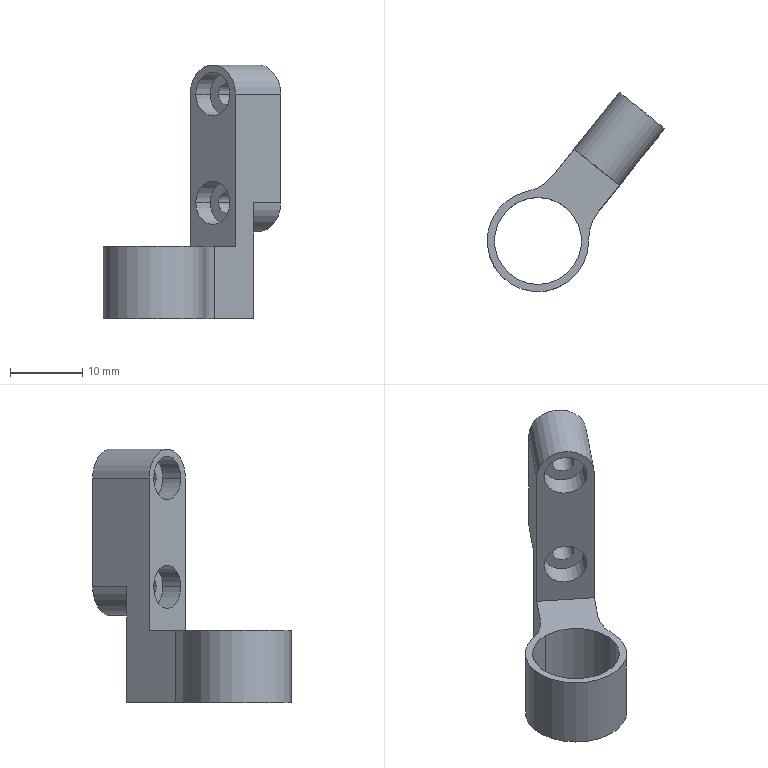Part | SolidWorks | features BaseBody 1 | 1 solid | 24 faces | box 24.488 x 27.462 x 35 mm | volume 2773 mm3 | cylinder 15 | plane 9 | commonest cylinder face diameters 3 x4 6 x4 12 x4 8 x2 14 x1
STEP:
#1=CARTESIAN_POINT('',(534.952,-197.215,297.045));
#2=VERTEX_POINT('',#1);
#3=CARTESIAN_POINT('',(534.952,-209.215,297.045));
#4=VERTEX_POINT('',#3);
#5=CARTESIAN_POINT('',(534.952,-203.215,297.045));
#6=DIRECTION('',(0.000000001,-0.000000003,1.));
#7=DIRECTION('',(0.,-1.,-0.000000003));
#8=AXIS2_PLACEMENT_3D('',#5,#6,#7);
#9=CIRCLE('',#8,6.);
#10=EDGE_CURVE('',#2,#4,#9,.T.);
#11=ORIENTED_EDGE('',*,*,#10,.F.);
#12=CARTESIAN_POINT('',(534.952,-197.215,307.045));
#13=VERTEX_POINT('',#12);
#14=CARTESIAN_POINT('',(534.952,-197.215,307.045));
#15=DIRECTION('',(0.000000001,-0.000000003,1.));
#16=VECTOR('',#15,1000.);
#17=LINE('',#14,#16);
#18=EDGE_CURVE('',#2,#13,#17,.T.);
#19=ORIENTED_EDGE('',*,*,#18,.T.);
#20=CARTESIAN_POINT('',(534.952,-209.215,307.045));
#21=VERTEX_POINT('',#20);
#22=CARTESIAN_POINT('',(534.952,-203.215,307.045));
#23=DIRECTION('',(-0.000000001,0.000000003,-1.));
#24=DIRECTION('',(0.,-1.,-0.000000003));
#25=AXIS2_PLACEMENT_3D('',#22,#23,#24);
#26=CIRCLE('',#25,6.);
#27=EDGE_CURVE('',#21,#13,#26,.T.);
#28=ORIENTED_EDGE('',*,*,#27,.F.);
#29=CARTESIAN_POINT('',(534.952,-209.215,307.045));
#30=DIRECTION('',(0.000000001,-0.000000003,1.));
#31=VECTOR('',#30,1000.);
#32=LINE('',#29,#31);
#33=EDGE_CURVE('',#4,#21,#32,.T.);
#34=ORIENTED_EDGE('',*,*,#33,.F.);
#35=EDGE_LOOP('',(#11,#19,#28,#34));
#36=FACE_OUTER_BOUND('',#35,.T.);
#37=CARTESIAN_POINT('',(534.952,-203.215,307.045));
#38=DIRECTION('',(0.000000001,-0.000000003,1.));
#39=DIRECTION('',(0.,-1.,-0.000000003));
#40=AXIS2_PLACEMENT_3D('',#37,#38,#39);
#41=CYLINDRICAL_SURFACE('',#40,6.);
#42=ADVANCED_FACE('',(#36),#41,.F.);
#43=CARTESIAN_POINT('',(542.711,-188.709,313.045));
#44=VERTEX_POINT('',#43);
#45=CARTESIAN_POINT('',(547.397,-192.455,313.045));
#46=VERTEX_POINT('',#45);
#47=CARTESIAN_POINT('',(545.054,-190.582,313.045));
#48=DIRECTION('',(-0.6245,-0.781,-0.000000002));
#49=DIRECTION('',(0.781,-0.6245,0.));
#50=AXIS2_PLACEMENT_3D('',#47,#48,#49);
#51=CIRCLE('',#50,3.);
#52=EDGE_CURVE('',#44,#46,#51,.T.);
#53=ORIENTED_EDGE('',*,*,#52,.F.);
#54=CARTESIAN_POINT('',(540.728,-191.188,313.045));
#55=VERTEX_POINT('',#54);
#56=CARTESIAN_POINT('',(541.719,-189.948,313.045));
#57=DIRECTION('',(-0.6245,-0.781,-0.000000002));
#58=VECTOR('',#57,1000.);
#59=LINE('',#56,#58);
#60=EDGE_CURVE('',#44,#55,#59,.T.);
#61=ORIENTED_EDGE('',*,*,#60,.T.);
#62=CARTESIAN_POINT('',(545.414,-194.935,313.045));
#63=VERTEX_POINT('',#62);
#64=CARTESIAN_POINT('',(543.071,-193.062,313.045));
#65=DIRECTION('',(0.6245,0.781,0.000000002));
#66=DIRECTION('',(0.781,-0.6245,0.));
#67=AXIS2_PLACEMENT_3D('',#64,#65,#66);
#68=CIRCLE('',#67,3.);
#69=EDGE_CURVE('',#63,#55,#68,.T.);
#70=ORIENTED_EDGE('',*,*,#69,.F.);
#71=CARTESIAN_POINT('',(546.405,-193.695,313.045));
#72=DIRECTION('',(-0.6245,-0.781,-0.000000002));
#73=VECTOR('',#72,1000.);
#74=LINE('',#71,#73);
#75=EDGE_CURVE('',#46,#63,#74,.T.);
#76=ORIENTED_EDGE('',*,*,#75,.F.);
#77=EDGE_LOOP('',(#53,#61,#70,#76));
#78=FACE_OUTER_BOUND('',#77,.T.);
#79=CARTESIAN_POINT('',(544.062,-191.822,313.045));
#80=DIRECTION('',(-0.6245,-0.781,-0.000000002));
#81=DIRECTION('',(0.781,-0.6245,0.));
#82=AXIS2_PLACEMENT_3D('',#79,#80,#81);
#83=CYLINDRICAL_SURFACE('',#82,3.);
#84=ADVANCED_FACE('',(#78),#83,.F.);
#85=CARTESIAN_POINT('',(542.711,-188.709,328.045));
#86=VERTEX_POINT('',#85);
#87=CARTESIAN_POINT('',(547.397,-192.455,328.045));
#88=VERTEX_POINT('',#87);
#89=CARTESIAN_POINT('',(545.054,-190.582,328.045));
#90=DIRECTION('',(-0.6245,-0.781,-0.000000002));
#91=DIRECTION('',(0.781,-0.6245,0.));
#92=AXIS2_PLACEMENT_3D('',#89,#90,#91);
#93=CIRCLE('',#92,3.);
#94=EDGE_CURVE('',#86,#88,#93,.T.);
#95=ORIENTED_EDGE('',*,*,#94,.F.);
#96=CARTESIAN_POINT('',(540.728,-191.188,328.045));
#97=VERTEX_POINT('',#96);
#98=CARTESIAN_POINT('',(541.719,-189.948,328.045));
#99=DIRECTION('',(-0.6245,-0.781,-0.000000002));
#100=VECTOR('',#99,1000.);
#101=LINE('',#98,#100);
#102=EDGE_CURVE('',#86,#97,#101,.T.);
#103=ORIENTED_EDGE('',*,*,#102,.T.);
#104=CARTESIAN_POINT('',(545.414,-194.935,328.045));
#105=VERTEX_POINT('',#104);
#106=CARTESIAN_POINT('',(543.071,-193.062,328.045));
#107=DIRECTION('',(0.6245,0.781,0.000000002));
#108=DIRECTION('',(0.781,-0.6245,0.));
#109=AXIS2_PLACEMENT_3D('',#106,#107,#108);
#110=CIRCLE('',#109,3.);
#111=EDGE_CURVE('',#105,#97,#110,.T.);
#112=ORIENTED_EDGE('',*,*,#111,.F.);
#113=CARTESIAN_POINT('',(546.405,-193.695,328.045));
#114=DIRECTION('',(-0.6245,-0.781,-0.000000002));
#115=VECTOR('',#114,1000.);
#116=LINE('',#113,#115);
#117=EDGE_CURVE('',#88,#105,#116,.T.);
#118=ORIENTED_EDGE('',*,*,#117,.F.);
#119=EDGE_LOOP('',(#95,#103,#112,#118));
#120=FACE_OUTER_BOUND('',#119,.T.);
#121=CARTESIAN_POINT('',(544.062,-191.822,328.045));
#122=DIRECTION('',(-0.6245,-0.781,-0.000000002));
#123=DIRECTION('',(0.781,-0.6245,0.));
#124=AXIS2_PLACEMENT_3D('',#121,#122,#123);
#125=CYLINDRICAL_SURFACE('',#124,3.);
#126=ADVANCED_FACE('',(#120),#125,.F.);
#127=CARTESIAN_POINT('',(548.144,-184.315,313.045));
#128=VERTEX_POINT('',#127);
#129=CARTESIAN_POINT('',(550.487,-186.188,313.045));
#130=VERTEX_POINT('',#129);
#131=CARTESIAN_POINT('',(549.316,-185.251,313.045));
#132=DIRECTION('',(-0.6245,-0.781,-0.000000002));
#133=DIRECTION('',(0.781,-0.6245,0.));
#134=AXIS2_PLACEMENT_3D('',#131,#132,#133);
#135=CIRCLE('',#134,1.5);
#136=EDGE_CURVE('',#128,#130,#135,.T.);
#137=ORIENTED_EDGE('',*,*,#136,.F.);
#138=CARTESIAN_POINT('',(543.882,-189.645,313.045));
#139=VERTEX_POINT('',#138);
#140=CARTESIAN_POINT('',(547.887,-184.637,313.045));
#141=DIRECTION('',(-0.6245,-0.781,-0.000000002));
#142=VECTOR('',#141,1000.);
#143=LINE('',#140,#142);
#144=EDGE_CURVE('',#128,#139,#143,.T.);
#145=ORIENTED_EDGE('',*,*,#144,.T.);
#146=CARTESIAN_POINT('',(546.225,-191.519,313.045));
#147=VERTEX_POINT('',#146);
#148=CARTESIAN_POINT('',(545.054,-190.582,313.045));
#149=DIRECTION('',(0.6245,0.781,0.000000002));
#150=DIRECTION('',(0.781,-0.6245,0.));
#151=AXIS2_PLACEMENT_3D('',#148,#149,#150);
#152=CIRCLE('',#151,1.5);
#153=EDGE_CURVE('',#147,#139,#152,.T.);
#154=ORIENTED_EDGE('',*,*,#153,.F.);
#155=CARTESIAN_POINT('',(550.23,-186.51,313.045));
#156=DIRECTION('',(-0.6245,-0.781,-0.000000002));
#157=VECTOR('',#156,1000.);
#158=LINE('',#155,#157);
#159=EDGE_CURVE('',#130,#147,#158,.T.);
#160=ORIENTED_EDGE('',*,*,#159,.F.);
#161=EDGE_LOOP('',(#137,#145,#154,#160));
#162=FACE_OUTER_BOUND('',#161,.T.);
#163=CARTESIAN_POINT('',(549.058,-185.574,313.045));
#164=DIRECTION('',(-0.6245,-0.781,-0.000000002));
#165=DIRECTION('',(0.781,-0.6245,0.));
#166=AXIS2_PLACEMENT_3D('',#163,#164,#165);
#167=CYLINDRICAL_SURFACE('',#166,1.5);
#168=ADVANCED_FACE('',(#162),#167,.F.);
#169=CARTESIAN_POINT('',(548.144,-184.315,328.045));
#170=VERTEX_POINT('',#169);
#171=CARTESIAN_POINT('',(550.487,-186.188,328.045));
#172=VERTEX_POINT('',#171);
#173=CARTESIAN_POINT('',(549.316,-185.251,328.045));
#174=DIRECTION('',(-0.6245,-0.781,-0.000000002));
#175=DIRECTION('',(0.781,-0.6245,0.));
#176=AXIS2_PLACEMENT_3D('',#173,#174,#175);
#177=CIRCLE('',#176,1.5);
#178=EDGE_CURVE('',#170,#172,#177,.T.);
#179=ORIENTED_EDGE('',*,*,#178,.F.);
#180=CARTESIAN_POINT('',(543.882,-189.645,328.045));
#181=VERTEX_POINT('',#180);
#182=CARTESIAN_POINT('',(547.887,-184.637,328.045));
#183=DIRECTION('',(-0.6245,-0.781,-0.000000002));
#184=VECTOR('',#183,1000.);
#185=LINE('',#182,#184);
#186=EDGE_CURVE('',#170,#181,#185,.T.);
#187=ORIENTED_EDGE('',*,*,#186,.T.);
#188=CARTESIAN_POINT('',(546.225,-191.519,328.045));
#189=VERTEX_POINT('',#188);
#190=CARTESIAN_POINT('',(545.054,-190.582,328.045));
#191=DIRECTION('',(0.6245,0.781,0.000000002));
#192=DIRECTION('',(0.781,-0.6245,0.));
#193=AXIS2_PLACEMENT_3D('',#190,#191,#192);
#194=CIRCLE('',#193,1.5);
#195=EDGE_CURVE('',#189,#181,#194,.T.);
#196=ORIENTED_EDGE('',*,*,#195,.F.);
#197=CARTESIAN_POINT('',(550.23,-186.51,328.045));
#198=DIRECTION('',(-0.6245,-0.781,-0.000000002));
#199=VECTOR('',#198,1000.);
#200=LINE('',#197,#199);
#201=EDGE_CURVE('',#172,#189,#200,.T.);
#202=ORIENTED_EDGE('',*,*,#201,.F.);
#203=EDGE_LOOP('',(#179,#187,#196,#202));
#204=FACE_OUTER_BOUND('',#203,.T.);
#205=CARTESIAN_POINT('',(549.058,-185.574,328.045));
#206=DIRECTION('',(-0.6245,-0.781,-0.000000002));
#207=DIRECTION('',(0.781,-0.6245,0.));
#208=AXIS2_PLACEMENT_3D('',#205,#206,#207);
#209=CYLINDRICAL_SURFACE('',#208,1.5);
#210=ADVANCED_FACE('',(#204),#209,.F.);
#211=CARTESIAN_POINT('',(546.195,-195.56,328.045));
#212=VERTEX_POINT('',#211);
#213=CARTESIAN_POINT('',(546.195,-195.56,307.045));
#214=VERTEX_POINT('',#213);
#215=CARTESIAN_POINT('',(546.195,-195.56,332.045));
#216=DIRECTION('',(-0.000000002,0.000000002,-1.));
#217=VECTOR('',#216,1000.);
#218=LINE('',#215,#217);
#219=EDGE_CURVE('',#212,#214,#218,.T.);
#220=ORIENTED_EDGE('',*,*,#219,.T.);
#221=CARTESIAN_POINT('',(543.264,-199.225,307.045));
#222=VERTEX_POINT('',#221);
#223=CARTESIAN_POINT('',(546.195,-195.56,307.045));
#224=DIRECTION('',(-0.6245,-0.781,0.));
#225=VECTOR('',#224,1000.);
#226=LINE('',#223,#225);
#227=EDGE_CURVE('',#214,#222,#226,.T.);
#228=ORIENTED_EDGE('',*,*,#227,.T.);
#229=CARTESIAN_POINT('',(543.264,-199.225,297.045));
#230=VERTEX_POINT('',#229);
#231=CARTESIAN_POINT('',(543.264,-199.225,332.045));
#232=DIRECTION('',(-0.000000002,0.000000002,-1.));
#233=VECTOR('',#232,1000.);
#234=LINE('',#231,#233);
#235=EDGE_CURVE('',#222,#230,#234,.T.);
#236=ORIENTED_EDGE('',*,*,#235,.T.);
#237=CARTESIAN_POINT('',(548.693,-192.436,297.045));
#238=VERTEX_POINT('',#237);
#239=CARTESIAN_POINT('',(546.195,-195.56,297.045));
#240=DIRECTION('',(0.6245,0.781,0.));
#241=VECTOR('',#240,1000.);
#242=LINE('',#239,#241);
#243=EDGE_CURVE('',#230,#238,#242,.T.);
#244=ORIENTED_EDGE('',*,*,#243,.T.);
#245=CARTESIAN_POINT('',(548.693,-192.436,313.045));
#246=VERTEX_POINT('',#245);
#247=CARTESIAN_POINT('',(548.693,-192.436,332.045));
#248=DIRECTION('',(0.000000002,-0.000000002,1.));
#249=VECTOR('',#248,1000.);
#250=LINE('',#247,#249);
#251=EDGE_CURVE('',#238,#246,#250,.T.);
#252=ORIENTED_EDGE('',*,*,#251,.T.);
#253=CARTESIAN_POINT('',(552.44,-187.749,313.045));
#254=VERTEX_POINT('',#253);
#255=CARTESIAN_POINT('',(546.195,-195.56,313.045));
#256=DIRECTION('',(0.6245,0.781,0.));
#257=VECTOR('',#256,1000.);
#258=LINE('',#255,#257);
#259=EDGE_CURVE('',#246,#254,#258,.T.);
#260=ORIENTED_EDGE('',*,*,#259,.T.);
#261=CARTESIAN_POINT('',(552.44,-187.749,328.045));
#262=VERTEX_POINT('',#261);
#263=CARTESIAN_POINT('',(552.44,-187.749,332.045));
#264=DIRECTION('',(0.000000002,-0.000000002,1.));
#265=VECTOR('',#264,1000.);
#266=LINE('',#263,#265);
#267=EDGE_CURVE('',#254,#262,#266,.T.);
#268=ORIENTED_EDGE('',*,*,#267,.T.);
#269=CARTESIAN_POINT('',(546.195,-195.56,328.045));
#270=DIRECTION('',(-0.6245,-0.781,0.));
#271=VECTOR('',#270,1000.);
#272=LINE('',#269,#271);
#273=EDGE_CURVE('',#262,#212,#272,.T.);
#274=ORIENTED_EDGE('',*,*,#273,.T.);
#275=EDGE_LOOP('',(#220,#228,#236,#244,#252,#260,#268,#274));
#276=FACE_OUTER_BOUND('',#275,.T.);
#277=CARTESIAN_POINT('',(546.195,-195.56,332.045));
#278=DIRECTION('',(0.781,-0.6245,-0.000000003));
#279=DIRECTION('',(0.6245,0.781,0.));
#280=AXIS2_PLACEMENT_3D('',#277,#278,#279);
#281=PLANE('',#280);
#282=ADVANCED_FACE('',(#276),#281,.T.);
#283=ORIENTED_EDGE('',*,*,#227,.F.);
#284=CARTESIAN_POINT('',(539.947,-190.564,307.045));
#285=VERTEX_POINT('',#284);
#286=CARTESIAN_POINT('',(546.195,-195.56,307.045));
#287=DIRECTION('',(-0.781,0.6245,0.000000003));
#288=VECTOR('',#287,1000.);
#289=LINE('',#286,#288);
#290=EDGE_CURVE('',#214,#285,#289,.T.);
#291=ORIENTED_EDGE('',*,*,#290,.T.);
#292=CARTESIAN_POINT('',(537.016,-194.229,307.045));
#293=VERTEX_POINT('',#292);
#294=CARTESIAN_POINT('',(539.947,-190.564,307.045));
#295=DIRECTION('',(-0.6245,-0.781,-0.000000002));
#296=VECTOR('',#295,1000.);
#297=LINE('',#294,#296);
#298=EDGE_CURVE('',#285,#293,#297,.T.);
#299=ORIENTED_EDGE('',*,*,#298,.T.);
#300=CARTESIAN_POINT('',(533.54,-196.359,307.045));
#301=VERTEX_POINT('',#300);
#302=CARTESIAN_POINT('',(532.33,-190.482,307.045));
#303=DIRECTION('',(-0.000000001,0.000000003,-1.));
#304=DIRECTION('',(0.,-1.,-0.000000003));
#305=AXIS2_PLACEMENT_3D('',#302,#303,#304);
#306=CIRCLE('',#305,6.);
#307=EDGE_CURVE('',#293,#301,#306,.T.);
#308=ORIENTED_EDGE('',*,*,#307,.T.);
#309=CARTESIAN_POINT('',(541.951,-203.084,307.045));
#310=VERTEX_POINT('',#309);
#311=CARTESIAN_POINT('',(534.952,-203.215,307.045));
#312=DIRECTION('',(0.000000001,-0.000000003,1.));
#313=DIRECTION('',(0.,1.,0.000000003));
#314=AXIS2_PLACEMENT_3D('',#311,#312,#313);
#315=CIRCLE('',#314,7.);
#316=EDGE_CURVE('',#301,#310,#315,.T.);
#317=ORIENTED_EDGE('',*,*,#316,.T.);
#318=CARTESIAN_POINT('',(547.95,-202.972,307.045));
#319=DIRECTION('',(-0.000000001,0.000000003,-1.));
#320=DIRECTION('',(0.,-1.,-0.000000003));
#321=AXIS2_PLACEMENT_3D('',#318,#319,#320);
#322=CIRCLE('',#321,6.);
#323=EDGE_CURVE('',#310,#222,#322,.T.);
#324=ORIENTED_EDGE('',*,*,#323,.T.);
#325=EDGE_LOOP('',(#283,#291,#299,#308,#317,#324));
#326=FACE_OUTER_BOUND('',#325,.T.);
#327=ORIENTED_EDGE('',*,*,#27,.T.);
#328=CARTESIAN_POINT('',(534.952,-203.215,307.045));
#329=DIRECTION('',(-0.000000001,0.000000003,-1.));
#330=DIRECTION('',(0.,-1.,-0.000000003));
#331=AXIS2_PLACEMENT_3D('',#328,#329,#330);
#332=CIRCLE('',#331,6.);
#333=EDGE_CURVE('',#13,#21,#332,.T.);
#334=ORIENTED_EDGE('',*,*,#333,.T.);
#335=EDGE_LOOP('',(#327,#334));
#336=FACE_BOUND('',#335,.T.);
#337=CARTESIAN_POINT('',(537.604,-188.69,307.045));
#338=DIRECTION('',(0.000000001,-0.000000003,1.));
#339=DIRECTION('',(0.,-1.,-0.000000003));
#340=AXIS2_PLACEMENT_3D('',#337,#338,#339);
#341=PLANE('',#340);
#342=ADVANCED_FACE('',(#326,#336),#341,.T.);
#343=CARTESIAN_POINT('',(539.947,-190.564,328.045));
#344=VERTEX_POINT('',#343);
#345=CARTESIAN_POINT('',(543.071,-193.062,328.045));
#346=DIRECTION('',(-0.6245,-0.781,-0.000000002));
#347=DIRECTION('',(-0.781,0.6245,0.));
#348=AXIS2_PLACEMENT_3D('',#345,#346,#347);
#349=CIRCLE('',#348,4.);
#350=EDGE_CURVE('',#212,#344,#349,.T.);
#351=ORIENTED_EDGE('',*,*,#350,.T.);
#352=CARTESIAN_POINT('',(539.947,-190.564,332.045));
#353=DIRECTION('',(0.000000001,0.000000002,-1.));
#354=VECTOR('',#353,1000.);
#355=LINE('',#352,#354);
#356=EDGE_CURVE('',#344,#285,#355,.T.);
#357=ORIENTED_EDGE('',*,*,#356,.T.);
#358=ORIENTED_EDGE('',*,*,#290,.F.);
#359=ORIENTED_EDGE('',*,*,#219,.F.);
#360=EDGE_LOOP('',(#351,#357,#358,#359));
#361=FACE_OUTER_BOUND('',#360,.T.);
#362=ORIENTED_EDGE('',*,*,#69,.T.);
#363=CARTESIAN_POINT('',(543.071,-193.062,313.045));
#364=DIRECTION('',(0.6245,0.781,0.000000002));
#365=DIRECTION('',(0.781,-0.6245,0.));
#366=AXIS2_PLACEMENT_3D('',#363,#364,#365);
#367=CIRCLE('',#366,3.);
#368=EDGE_CURVE('',#55,#63,#367,.T.);
#369=ORIENTED_EDGE('',*,*,#368,.T.);
#370=EDGE_LOOP('',(#362,#369));
#371=FACE_BOUND('',#370,.T.);
#372=ORIENTED_EDGE('',*,*,#111,.T.);
#373=CARTESIAN_POINT('',(543.071,-193.062,328.045));
#374=DIRECTION('',(0.6245,0.781,0.000000002));
#375=DIRECTION('',(0.781,-0.6245,0.));
#376=AXIS2_PLACEMENT_3D('',#373,#374,#375);
#377=CIRCLE('',#376,3.);
#378=EDGE_CURVE('',#97,#105,#377,.T.);
#379=ORIENTED_EDGE('',*,*,#378,.T.);
#380=EDGE_LOOP('',(#372,#379));
#381=FACE_BOUND('',#380,.T.);
#382=CARTESIAN_POINT('',(539.947,-190.564,332.045));
#383=DIRECTION('',(-0.6245,-0.781,-0.000000002));
#384=DIRECTION('',(0.781,-0.6245,0.));
#385=AXIS2_PLACEMENT_3D('',#382,#383,#384);
#386=PLANE('',#385);
#387=ADVANCED_FACE('',(#361,#371,#381),#386,.T.);
#388=ORIENTED_EDGE('',*,*,#273,.F.);
#389=CARTESIAN_POINT('',(546.192,-182.753,328.045));
#390=VERTEX_POINT('',#389);
#391=CARTESIAN_POINT('',(549.316,-185.251,328.045));
#392=DIRECTION('',(-0.6245,-0.781,-0.000000002));
#393=DIRECTION('',(-0.781,0.6245,0.));
#394=AXIS2_PLACEMENT_3D('',#391,#392,#393);
#395=CIRCLE('',#394,4.);
#396=EDGE_CURVE('',#262,#390,#395,.T.);
#397=ORIENTED_EDGE('',*,*,#396,.T.);
#398=CARTESIAN_POINT('',(546.192,-182.753,328.045));
#399=DIRECTION('',(0.6245,0.781,0.));
#400=VECTOR('',#399,1000.);
#401=LINE('',#398,#400);
#402=EDGE_CURVE('',#344,#390,#401,.T.);
#403=ORIENTED_EDGE('',*,*,#402,.F.);
#404=ORIENTED_EDGE('',*,*,#350,.F.);
#405=EDGE_LOOP('',(#388,#397,#403,#404));
#406=FACE_OUTER_BOUND('',#405,.T.);
#407=CARTESIAN_POINT('',(547.755,-187.204,328.045));
#408=DIRECTION('',(0.6245,0.781,0.000000002));
#409=DIRECTION('',(-0.781,0.6245,0.));
#410=AXIS2_PLACEMENT_3D('',#407,#408,#409);
#411=CYLINDRICAL_SURFACE('',#410,4.);
#412=ADVANCED_FACE('',(#406),#411,.T.);
#413=ORIENTED_EDGE('',*,*,#267,.F.);
#414=CARTESIAN_POINT('',(546.192,-182.753,313.045));
#415=VERTEX_POINT('',#414);
#416=CARTESIAN_POINT('',(549.316,-185.251,313.045));
#417=DIRECTION('',(0.6245,0.781,0.000000002));
#418=DIRECTION('',(0.781,-0.6245,0.));
#419=AXIS2_PLACEMENT_3D('',#416,#417,#418);
#420=CIRCLE('',#419,4.);
#421=EDGE_CURVE('',#254,#415,#420,.T.);
#422=ORIENTED_EDGE('',*,*,#421,.T.);
#423=CARTESIAN_POINT('',(546.192,-182.753,332.045));
#424=DIRECTION('',(-0.000000001,-0.000000002,1.));
#425=VECTOR('',#424,1000.);
#426=LINE('',#423,#425);
#427=EDGE_CURVE('',#415,#390,#426,.T.);
#428=ORIENTED_EDGE('',*,*,#427,.T.);
#429=ORIENTED_EDGE('',*,*,#396,.F.);
#430=EDGE_LOOP('',(#413,#422,#428,#429));
#431=FACE_OUTER_BOUND('',#430,.T.);
#432=CARTESIAN_POINT('',(549.316,-185.251,313.045));
#433=DIRECTION('',(-0.6245,-0.781,-0.000000002));
#434=DIRECTION('',(0.781,-0.6245,0.));
#435=AXIS2_PLACEMENT_3D('',#432,#433,#434);
#436=CIRCLE('',#435,1.5);
#437=EDGE_CURVE('',#130,#128,#436,.T.);
#438=ORIENTED_EDGE('',*,*,#437,.T.);
#439=ORIENTED_EDGE('',*,*,#136,.T.);
#440=EDGE_LOOP('',(#438,#439));
#441=FACE_BOUND('',#440,.T.);
#442=CARTESIAN_POINT('',(549.316,-185.251,328.045));
#443=DIRECTION('',(-0.6245,-0.781,-0.000000002));
#444=DIRECTION('',(0.781,-0.6245,0.));
#445=AXIS2_PLACEMENT_3D('',#442,#443,#444);
#446=CIRCLE('',#445,1.5);
#447=EDGE_CURVE('',#172,#170,#446,.T.);
#448=ORIENTED_EDGE('',*,*,#447,.T.);
#449=ORIENTED_EDGE('',*,*,#178,.T.);
#450=EDGE_LOOP('',(#448,#449));
#451=FACE_BOUND('',#450,.T.);
#452=CARTESIAN_POINT('',(552.44,-187.749,332.045));
#453=DIRECTION('',(0.6245,0.781,0.000000002));
#454=DIRECTION('',(-0.781,0.6245,0.));
#455=AXIS2_PLACEMENT_3D('',#452,#453,#454);
#456=PLANE('',#455);
#457=ADVANCED_FACE('',(#431,#441,#451),#456,.T.);
#458=ORIENTED_EDGE('',*,*,#259,.F.);
#459=CARTESIAN_POINT('',(542.445,-187.44,313.045));
#460=VERTEX_POINT('',#459);
#461=CARTESIAN_POINT('',(545.569,-189.938,313.045));
#462=DIRECTION('',(0.6245,0.781,0.000000002));
#463=DIRECTION('',(0.781,-0.6245,0.));
#464=AXIS2_PLACEMENT_3D('',#461,#462,#463);
#465=CIRCLE('',#464,4.);
#466=EDGE_CURVE('',#246,#460,#465,.T.);
#467=ORIENTED_EDGE('',*,*,#466,.T.);
#468=CARTESIAN_POINT('',(546.192,-182.753,313.045));
#469=DIRECTION('',(-0.6245,-0.781,0.));
#470=VECTOR('',#469,1000.);
#471=LINE('',#468,#470);
#472=EDGE_CURVE('',#415,#460,#471,.T.);
#473=ORIENTED_EDGE('',*,*,#472,.F.);
#474=ORIENTED_EDGE('',*,*,#421,.F.);
#475=EDGE_LOOP('',(#458,#467,#473,#474));
#476=FACE_OUTER_BOUND('',#475,.T.);
#477=CARTESIAN_POINT('',(549.316,-185.251,313.045));
#478=DIRECTION('',(-0.6245,-0.781,-0.000000002));
#479=DIRECTION('',(0.781,-0.6245,0.));
#480=AXIS2_PLACEMENT_3D('',#477,#478,#479);
#481=CYLINDRICAL_SURFACE('',#480,4.);
#482=ADVANCED_FACE('',(#476),#481,.T.);
#483=CARTESIAN_POINT('',(542.445,-187.44,297.045));
#484=VERTEX_POINT('',#483);
#485=CARTESIAN_POINT('',(542.445,-187.44,290.545));
#486=DIRECTION('',(0.000000001,0.000000002,-1.));
#487=VECTOR('',#486,1000.);
#488=LINE('',#485,#487);
#489=EDGE_CURVE('',#460,#484,#488,.T.);
#490=ORIENTED_EDGE('',*,*,#489,.F.);
#491=ORIENTED_EDGE('',*,*,#466,.F.);
#492=ORIENTED_EDGE('',*,*,#251,.F.);
#493=CARTESIAN_POINT('',(545.531,-189.908,297.045));
#494=DIRECTION('',(0.781,-0.6245,0.));
#495=VECTOR('',#494,1000.);
#496=LINE('',#493,#495);
#497=EDGE_CURVE('',#484,#238,#496,.T.);
#498=ORIENTED_EDGE('',*,*,#497,.F.);
#499=EDGE_LOOP('',(#490,#491,#492,#498));
#500=FACE_OUTER_BOUND('',#499,.T.);
#501=CARTESIAN_POINT('',(545.531,-189.908,290.545));
#502=DIRECTION('',(-0.6245,-0.781,-0.000000002));
#503=DIRECTION('',(0.781,-0.6245,0.));
#504=AXIS2_PLACEMENT_3D('',#501,#502,#503);
#505=PLANE('',#504);
#506=ADVANCED_FACE('',(#500),#505,.F.);
#507=CARTESIAN_POINT('',(541.951,-203.084,297.045));
#508=VERTEX_POINT('',#507);
#509=CARTESIAN_POINT('',(533.54,-196.359,297.045));
#510=VERTEX_POINT('',#509);
#511=CARTESIAN_POINT('',(534.952,-203.215,297.045));
#512=DIRECTION('',(-0.000000001,0.000000003,-1.));
#513=DIRECTION('',(0.,1.,0.000000003));
#514=AXIS2_PLACEMENT_3D('',#511,#512,#513);
#515=CIRCLE('',#514,7.);
#516=EDGE_CURVE('',#508,#510,#515,.T.);
#517=ORIENTED_EDGE('',*,*,#516,.T.);
#518=CARTESIAN_POINT('',(537.016,-194.229,297.045));
#519=VERTEX_POINT('',#518);
#520=CARTESIAN_POINT('',(532.33,-190.482,297.045));
#521=DIRECTION('',(0.000000001,-0.000000003,1.));
#522=DIRECTION('',(0.,-1.,-0.000000003));
#523=AXIS2_PLACEMENT_3D('',#520,#521,#522);
#524=CIRCLE('',#523,6.);
#525=EDGE_CURVE('',#510,#519,#524,.T.);
#526=ORIENTED_EDGE('',*,*,#525,.T.);
#527=CARTESIAN_POINT('',(537.016,-194.229,297.045));
#528=DIRECTION('',(0.6245,0.781,0.000000002));
#529=VECTOR('',#528,1000.);
#530=LINE('',#527,#529);
#531=EDGE_CURVE('',#519,#484,#530,.T.);
#532=ORIENTED_EDGE('',*,*,#531,.T.);
#533=ORIENTED_EDGE('',*,*,#497,.T.);
#534=ORIENTED_EDGE('',*,*,#243,.F.);
#535=CARTESIAN_POINT('',(547.95,-202.972,297.045));
#536=DIRECTION('',(0.000000001,-0.000000003,1.));
#537=DIRECTION('',(0.,-1.,-0.000000003));
#538=AXIS2_PLACEMENT_3D('',#535,#536,#537);
#539=CIRCLE('',#538,6.);
#540=EDGE_CURVE('',#230,#508,#539,.T.);
#541=ORIENTED_EDGE('',*,*,#540,.T.);
#542=EDGE_LOOP('',(#517,#526,#532,#533,#534,#541));
#543=FACE_OUTER_BOUND('',#542,.T.);
#544=CARTESIAN_POINT('',(534.952,-203.215,297.045));
#545=DIRECTION('',(0.000000001,-0.000000003,1.));
#546=DIRECTION('',(0.,-1.,-0.000000003));
#547=AXIS2_PLACEMENT_3D('',#544,#545,#546);
#548=CIRCLE('',#547,6.);
#549=EDGE_CURVE('',#4,#2,#548,.T.);
#550=ORIENTED_EDGE('',*,*,#549,.T.);
#551=ORIENTED_EDGE('',*,*,#10,.T.);
#552=EDGE_LOOP('',(#550,#551));
#553=FACE_BOUND('',#552,.T.);
#554=CARTESIAN_POINT('',(546.193,-189.157,297.045));
#555=DIRECTION('',(-0.000000001,0.000000003,-1.));
#556=DIRECTION('',(0.,1.,0.000000003));
#557=AXIS2_PLACEMENT_3D('',#554,#555,#556);
#558=PLANE('',#557);
#559=ADVANCED_FACE('',(#543,#553),#558,.T.);
#560=ORIENTED_EDGE('',*,*,#540,.F.);
#561=ORIENTED_EDGE('',*,*,#235,.F.);
#562=ORIENTED_EDGE('',*,*,#323,.F.);
#563=CARTESIAN_POINT('',(541.951,-203.084,304.545));
#564=DIRECTION('',(0.000000001,-0.000000003,1.));
#565=VECTOR('',#564,1000.);
#566=LINE('',#563,#565);
#567=EDGE_CURVE('',#508,#310,#566,.T.);
#568=ORIENTED_EDGE('',*,*,#567,.F.);
#569=EDGE_LOOP('',(#560,#561,#562,#568));
#570=FACE_OUTER_BOUND('',#569,.T.);
#571=CARTESIAN_POINT('',(547.95,-202.972,304.545));
#572=DIRECTION('',(0.000000001,-0.000000003,1.));
#573=DIRECTION('',(0.,-1.,-0.000000003));
#574=AXIS2_PLACEMENT_3D('',#571,#572,#573);
#575=CYLINDRICAL_SURFACE('',#574,6.);
#576=ADVANCED_FACE('',(#570),#575,.F.);
#577=ORIENTED_EDGE('',*,*,#567,.T.);
#578=ORIENTED_EDGE('',*,*,#316,.F.);
#579=CARTESIAN_POINT('',(533.54,-196.359,304.545));
#580=DIRECTION('',(-0.000000001,0.000000003,-1.));
#581=VECTOR('',#580,1000.);
#582=LINE('',#579,#581);
#583=EDGE_CURVE('',#301,#510,#582,.T.);
#584=ORIENTED_EDGE('',*,*,#583,.T.);
#585=ORIENTED_EDGE('',*,*,#516,.F.);
#586=EDGE_LOOP('',(#577,#578,#584,#585));
#587=FACE_OUTER_BOUND('',#586,.T.);
#588=CARTESIAN_POINT('',(534.952,-203.215,304.545));
#589=DIRECTION('',(-0.000000001,0.000000003,-1.));
#590=DIRECTION('',(0.,1.,0.000000003));
#591=AXIS2_PLACEMENT_3D('',#588,#589,#590);
#592=CYLINDRICAL_SURFACE('',#591,7.);
#593=ADVANCED_FACE('',(#587),#592,.T.);
#594=ORIENTED_EDGE('',*,*,#525,.F.);
#595=ORIENTED_EDGE('',*,*,#583,.F.);
#596=ORIENTED_EDGE('',*,*,#307,.F.);
#597=CARTESIAN_POINT('',(537.016,-194.229,304.545));
#598=DIRECTION('',(0.000000001,-0.000000003,1.));
#599=VECTOR('',#598,1000.);
#600=LINE('',#597,#599);
#601=EDGE_CURVE('',#519,#293,#600,.T.);
#602=ORIENTED_EDGE('',*,*,#601,.F.);
#603=EDGE_LOOP('',(#594,#595,#596,#602));
#604=FACE_OUTER_BOUND('',#603,.T.);
#605=CARTESIAN_POINT('',(532.33,-190.482,304.545));
#606=DIRECTION('',(0.000000001,-0.000000003,1.));
#607=DIRECTION('',(0.,-1.,-0.000000003));
#608=AXIS2_PLACEMENT_3D('',#605,#606,#607);
#609=CYLINDRICAL_SURFACE('',#608,6.);
#610=ADVANCED_FACE('',(#604),#609,.F.);
#611=ORIENTED_EDGE('',*,*,#489,.T.);
#612=ORIENTED_EDGE('',*,*,#531,.F.);
#613=ORIENTED_EDGE('',*,*,#601,.T.);
#614=ORIENTED_EDGE('',*,*,#298,.F.);
#615=ORIENTED_EDGE('',*,*,#356,.F.);
#616=ORIENTED_EDGE('',*,*,#402,.T.);
#617=ORIENTED_EDGE('',*,*,#427,.F.);
#618=ORIENTED_EDGE('',*,*,#472,.T.);
#619=EDGE_LOOP('',(#611,#612,#613,#614,#615,#616,#617,#618));
#620=FACE_OUTER_BOUND('',#619,.T.);
#621=CARTESIAN_POINT('',(546.192,-182.753,332.045));
#622=DIRECTION('',(-0.781,0.6245,0.000000003));
#623=DIRECTION('',(-0.6245,-0.781,0.));
#624=AXIS2_PLACEMENT_3D('',#621,#622,#623);
#625=PLANE('',#624);
#626=ADVANCED_FACE('',(#620),#625,.T.);
#627=ORIENTED_EDGE('',*,*,#18,.F.);
#628=ORIENTED_EDGE('',*,*,#549,.F.);
#629=ORIENTED_EDGE('',*,*,#33,.T.);
#630=ORIENTED_EDGE('',*,*,#333,.F.);
#631=EDGE_LOOP('',(#627,#628,#629,#630));
#632=FACE_OUTER_BOUND('',#631,.T.);
#633=CARTESIAN_POINT('',(534.952,-203.215,307.045));
#634=DIRECTION('',(0.000000001,-0.000000003,1.));
#635=DIRECTION('',(0.,-1.,-0.000000003));
#636=AXIS2_PLACEMENT_3D('',#633,#634,#635);
#637=CYLINDRICAL_SURFACE('',#636,6.);
#638=ADVANCED_FACE('',(#632),#637,.F.);
#639=ORIENTED_EDGE('',*,*,#60,.F.);
#640=CARTESIAN_POINT('',(545.054,-190.582,313.045));
#641=DIRECTION('',(-0.6245,-0.781,-0.000000002));
#642=DIRECTION('',(0.781,-0.6245,0.));
#643=AXIS2_PLACEMENT_3D('',#640,#641,#642);
#644=CIRCLE('',#643,3.);
#645=EDGE_CURVE('',#46,#44,#644,.T.);
#646=ORIENTED_EDGE('',*,*,#645,.F.);
#647=ORIENTED_EDGE('',*,*,#75,.T.);
#648=ORIENTED_EDGE('',*,*,#368,.F.);
#649=EDGE_LOOP('',(#639,#646,#647,#648));
#650=FACE_OUTER_BOUND('',#649,.T.);
#651=CARTESIAN_POINT('',(544.062,-191.822,313.045));
#652=DIRECTION('',(-0.6245,-0.781,-0.000000002));
#653=DIRECTION('',(0.781,-0.6245,0.));
#654=AXIS2_PLACEMENT_3D('',#651,#652,#653);
#655=CYLINDRICAL_SURFACE('',#654,3.);
#656=ADVANCED_FACE('',(#650),#655,.F.);
#657=ORIENTED_EDGE('',*,*,#102,.F.);
#658=CARTESIAN_POINT('',(545.054,-190.582,328.045));
#659=DIRECTION('',(-0.6245,-0.781,-0.000000002));
#660=DIRECTION('',(0.781,-0.6245,0.));
#661=AXIS2_PLACEMENT_3D('',#658,#659,#660);
#662=CIRCLE('',#661,3.);
#663=EDGE_CURVE('',#88,#86,#662,.T.);
#664=ORIENTED_EDGE('',*,*,#663,.F.);
#665=ORIENTED_EDGE('',*,*,#117,.T.);
#666=ORIENTED_EDGE('',*,*,#378,.F.);
#667=EDGE_LOOP('',(#657,#664,#665,#666));
#668=FACE_OUTER_BOUND('',#667,.T.);
#669=CARTESIAN_POINT('',(544.062,-191.822,328.045));
#670=DIRECTION('',(-0.6245,-0.781,-0.000000002));
#671=DIRECTION('',(0.781,-0.6245,0.));
#672=AXIS2_PLACEMENT_3D('',#669,#670,#671);
#673=CYLINDRICAL_SURFACE('',#672,3.);
#674=ADVANCED_FACE('',(#668),#673,.F.);
#675=ORIENTED_EDGE('',*,*,#144,.F.);
#676=ORIENTED_EDGE('',*,*,#437,.F.);
#677=ORIENTED_EDGE('',*,*,#159,.T.);
#678=CARTESIAN_POINT('',(545.054,-190.582,313.045));
#679=DIRECTION('',(0.6245,0.781,0.000000002));
#680=DIRECTION('',(0.781,-0.6245,0.));
#681=AXIS2_PLACEMENT_3D('',#678,#679,#680);
#682=CIRCLE('',#681,1.5);
#683=EDGE_CURVE('',#139,#147,#682,.T.);
#684=ORIENTED_EDGE('',*,*,#683,.F.);
#685=EDGE_LOOP('',(#675,#676,#677,#684));
#686=FACE_OUTER_BOUND('',#685,.T.);
#687=CARTESIAN_POINT('',(549.058,-185.574,313.045));
#688=DIRECTION('',(-0.6245,-0.781,-0.000000002));
#689=DIRECTION('',(0.781,-0.6245,0.));
#690=AXIS2_PLACEMENT_3D('',#687,#688,#689);
#691=CYLINDRICAL_SURFACE('',#690,1.5);
#692=ADVANCED_FACE('',(#686),#691,.F.);
#693=ORIENTED_EDGE('',*,*,#186,.F.);
#694=ORIENTED_EDGE('',*,*,#447,.F.);
#695=ORIENTED_EDGE('',*,*,#201,.T.);
#696=CARTESIAN_POINT('',(545.054,-190.582,328.045));
#697=DIRECTION('',(0.6245,0.781,0.000000002));
#698=DIRECTION('',(0.781,-0.6245,0.));
#699=AXIS2_PLACEMENT_3D('',#696,#697,#698);
#700=CIRCLE('',#699,1.5);
#701=EDGE_CURVE('',#181,#189,#700,.T.);
#702=ORIENTED_EDGE('',*,*,#701,.F.);
#703=EDGE_LOOP('',(#693,#694,#695,#702));
#704=FACE_OUTER_BOUND('',#703,.T.);
#705=CARTESIAN_POINT('',(549.058,-185.574,328.045));
#706=DIRECTION('',(-0.6245,-0.781,-0.000000002));
#707=DIRECTION('',(0.781,-0.6245,0.));
#708=AXIS2_PLACEMENT_3D('',#705,#706,#707);
#709=CYLINDRICAL_SURFACE('',#708,1.5);
#710=ADVANCED_FACE('',(#704),#709,.F.);
#711=ORIENTED_EDGE('',*,*,#645,.T.);
#712=ORIENTED_EDGE('',*,*,#52,.T.);
#713=EDGE_LOOP('',(#711,#712));
#714=FACE_OUTER_BOUND('',#713,.T.);
#715=ORIENTED_EDGE('',*,*,#153,.T.);
#716=ORIENTED_EDGE('',*,*,#683,.T.);
#717=EDGE_LOOP('',(#715,#716));
#718=FACE_BOUND('',#717,.T.);
#719=CARTESIAN_POINT('',(546.811,-191.987,313.045));
#720=DIRECTION('',(0.6245,0.781,0.000000002));
#721=DIRECTION('',(-0.781,0.6245,0.));
#722=AXIS2_PLACEMENT_3D('',#719,#720,#721);
#723=PLANE('',#722);
#724=ADVANCED_FACE('',(#714,#718),#723,.F.);
#725=ORIENTED_EDGE('',*,*,#663,.T.);
#726=ORIENTED_EDGE('',*,*,#94,.T.);
#727=EDGE_LOOP('',(#725,#726));
#728=FACE_OUTER_BOUND('',#727,.T.);
#729=ORIENTED_EDGE('',*,*,#195,.T.);
#730=ORIENTED_EDGE('',*,*,#701,.T.);
#731=EDGE_LOOP('',(#729,#730));
#732=FACE_BOUND('',#731,.T.);
#733=CARTESIAN_POINT('',(546.811,-191.987,328.045));
#734=DIRECTION('',(0.6245,0.781,0.000000002));
#735=DIRECTION('',(-0.781,0.6245,0.));
#736=AXIS2_PLACEMENT_3D('',#733,#734,#735);
#737=PLANE('',#736);
#738=ADVANCED_FACE('',(#728,#732),#737,.F.);
#739=CLOSED_SHELL('',(#42,#84,#126,#168,#210,#282,#342,#387,#412,#457,#482,#506,#559,#576,#593,#610,#626,#638,#656,#674,#692,#710,#724,#738));
#740=MANIFOLD_SOLID_BREP('',#739);
#741=CARTESIAN_POINT('',(0.,0.,0.));
#742=DIRECTION('',(0.,0.,1.));
#743=DIRECTION('',(1.,0.,0.));
#744=AXIS2_PLACEMENT_3D('',#741,#742,#743);
#745=(LENGTH_UNIT()NAMED_UNIT(*)SI_UNIT(.MILLI.,.METRE.));
#746=UNCERTAINTY_MEASURE_WITH_UNIT(LENGTH_MEASURE(0.00001),#745,'','');
#747=(NAMED_UNIT(*)PLANE_ANGLE_UNIT()SI_UNIT($,.RADIAN.));
#748=(NAMED_UNIT(*)SI_UNIT($,.STERADIAN.)SOLID_ANGLE_UNIT());
#749=(GEOMETRIC_REPRESENTATION_CONTEXT(3)GLOBAL_UNCERTAINTY_ASSIGNED_CONTEXT((#746))GLOBAL_UNIT_ASSIGNED_CONTEXT((#745,#747,#748))REPRESENTATION_CONTEXT('',''));
#750=ADVANCED_BREP_SHAPE_REPRESENTATION('',(#740,#744),#749);